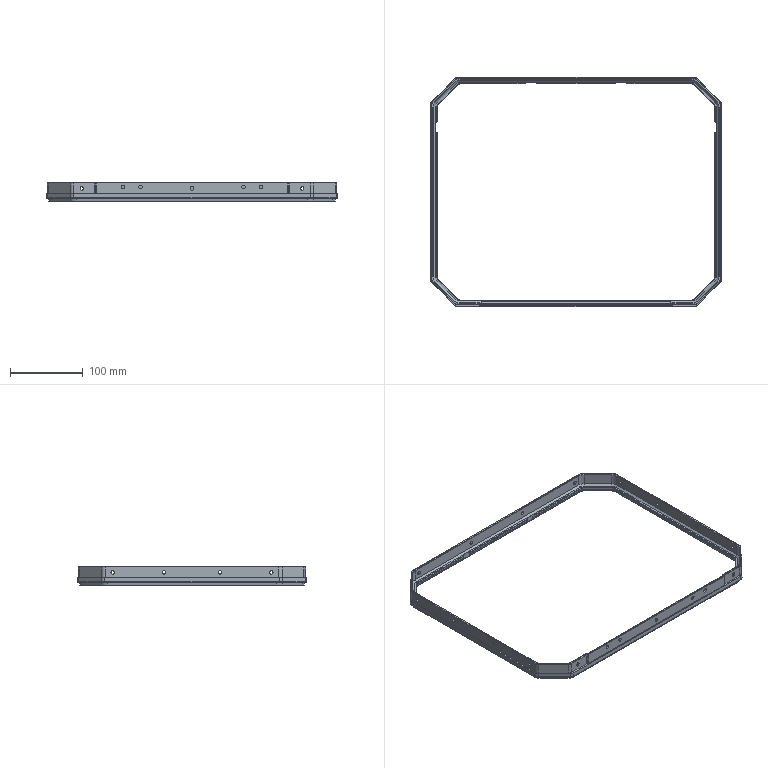Part | SolidWorks | features BaseBody 1 | 1 solid | 398 faces | box 400 x 315 x 26 mm | volume 132003 mm3 | cylinder 154 | plane 116 | torus 48 | cone 44 | spline 20 | sphere 16 | commonest cylinder face diameters 1 x60 4.9 x38 12 x16 5.2 x8 10.6 x8 13.6 x8